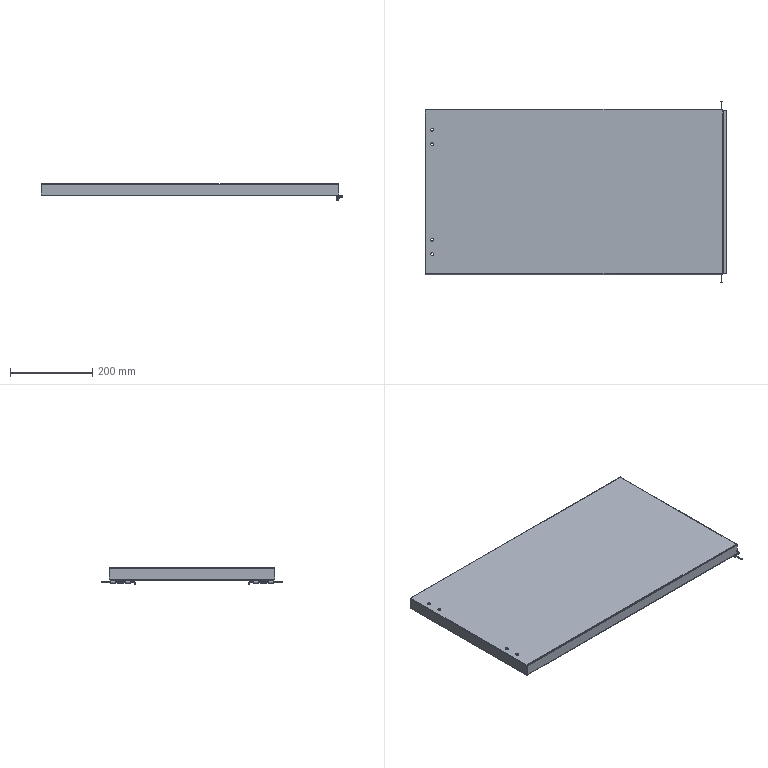Part | 5 solids | 145 faces | box 732.8 x 438.127 x 41 mm | volume 455793 mm3 | plane 76 | cylinder 51 | spline 14 | torus 4 | commonest cylinder face diameters 7 x11 1.473 x8 3 x8 3.6 x8 3.873 x8 7.6 x8